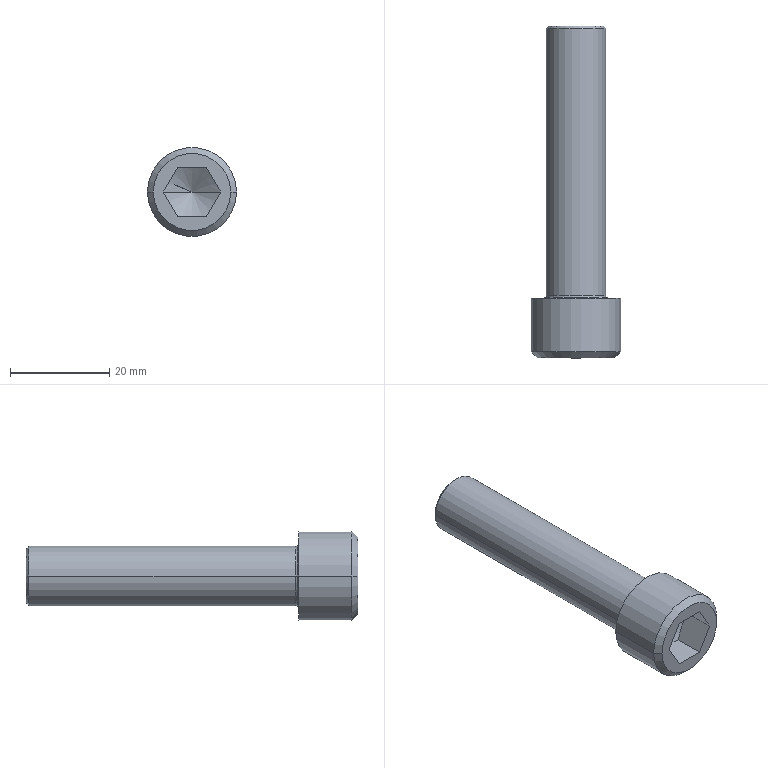Part | Creo | 1 solid | 23 faces | box 18 x 67 x 18 mm | volume 8601 mm3 | plane 9 | cone 6 | cylinder 4 | torus 4 | commonest cylinder face diameters 12 x2 18 x2
STEP:
#1=CARTESIAN_POINT('',(0.,0.,0.));
#2=DIRECTION('',(0.,0.,1.));
#3=DIRECTION('',(1.,0.,0.));
#4=AXIS2_PLACEMENT_3D('',#1,#2,#3);
#5=CARTESIAN_POINT('',(159.226,-292.,-52.5));
#6=VERTEX_POINT('',#5);
#7=CARTESIAN_POINT('',(162.113,-292.,-57.5));
#8=VERTEX_POINT('',#7);
#9=CARTESIAN_POINT('',(159.226,-292.,-52.5));
#10=CARTESIAN_POINT('',(159.361,-291.922,-52.733));
#11=CARTESIAN_POINT('',(159.631,-291.783,-53.201));
#12=CARTESIAN_POINT('',(160.043,-291.631,-53.914));
#13=CARTESIAN_POINT('',(160.46,-291.55,-54.636));
#14=CARTESIAN_POINT('',(160.878,-291.55,-55.36));
#15=CARTESIAN_POINT('',(161.296,-291.63,-56.084));
#16=CARTESIAN_POINT('',(161.707,-291.782,-56.796));
#17=CARTESIAN_POINT('',(161.978,-291.922,-57.266));
#18=CARTESIAN_POINT('',(162.113,-292.,-57.5));
#19=B_SPLINE_CURVE_WITH_KNOTS('',3,(#9,#10,#11,#12,#13,#14,#15,#16,#17,#18),.UNSPECIFIED.,.F.,.F.,(4,1,1,1,1,1,1,4),(0.,0.1429,0.2857,0.4286,0.5714,0.7143,0.8571,1.),.UNSPECIFIED.);
#20=EDGE_CURVE('',#6,#8,#19,.T.);
#21=ORIENTED_EDGE('',*,*,#20,.F.);
#22=CARTESIAN_POINT('',(165.,-288.667,-52.5));
#23=VERTEX_POINT('',#22);
#24=CARTESIAN_POINT('',(165.,-288.667,-52.5));
#25=DIRECTION('',(-0.866,-0.5,0.));
#26=VECTOR('',#25,6.667);
#27=LINE('',#24,#26);
#28=EDGE_CURVE('',#23,#6,#27,.T.);
#29=ORIENTED_EDGE('',*,*,#28,.F.);
#30=CARTESIAN_POINT('',(170.774,-292.,-52.5));
#31=VERTEX_POINT('',#30);
#32=CARTESIAN_POINT('',(165.,-288.667,-52.5));
#33=DIRECTION('',(0.866,-0.5,0.));
#34=VECTOR('',#33,6.667);
#35=LINE('',#32,#34);
#36=EDGE_CURVE('',#23,#31,#35,.T.);
#37=ORIENTED_EDGE('',*,*,#36,.T.);
#38=CARTESIAN_POINT('',(167.887,-292.,-57.5));
#39=VERTEX_POINT('',#38);
#40=CARTESIAN_POINT('',(167.887,-292.,-57.5));
#41=CARTESIAN_POINT('',(168.021,-291.922,-57.267));
#42=CARTESIAN_POINT('',(168.291,-291.783,-56.799));
#43=CARTESIAN_POINT('',(168.703,-291.631,-56.086));
#44=CARTESIAN_POINT('',(169.12,-291.55,-55.364));
#45=CARTESIAN_POINT('',(169.538,-291.55,-54.64));
#46=CARTESIAN_POINT('',(169.956,-291.63,-53.916));
#47=CARTESIAN_POINT('',(170.367,-291.782,-53.204));
#48=CARTESIAN_POINT('',(170.638,-291.922,-52.734));
#49=CARTESIAN_POINT('',(170.774,-292.,-52.5));
#50=B_SPLINE_CURVE_WITH_KNOTS('',3,(#40,#41,#42,#43,#44,#45,#46,#47,#48,#49),.UNSPECIFIED.,.F.,.F.,(4,1,1,1,1,1,1,4),(0.,0.1429,0.2857,0.4286,0.5714,0.7143,0.8571,1.),.UNSPECIFIED.);
#51=EDGE_CURVE('',#39,#31,#50,.T.);
#52=ORIENTED_EDGE('',*,*,#51,.F.);
#53=CARTESIAN_POINT('',(162.113,-292.,-57.5));
#54=CARTESIAN_POINT('',(162.381,-291.923,-57.5));
#55=CARTESIAN_POINT('',(162.919,-291.783,-57.5));
#56=CARTESIAN_POINT('',(163.745,-291.631,-57.5));
#57=CARTESIAN_POINT('',(164.581,-291.55,-57.5));
#58=CARTESIAN_POINT('',(165.416,-291.55,-57.5));
#59=CARTESIAN_POINT('',(166.25,-291.63,-57.5));
#60=CARTESIAN_POINT('',(167.077,-291.782,-57.5));
#61=CARTESIAN_POINT('',(167.618,-291.922,-57.5));
#62=CARTESIAN_POINT('',(167.887,-292.,-57.5));
#63=B_SPLINE_CURVE_WITH_KNOTS('',3,(#53,#54,#55,#56,#57,#58,#59,#60,#61,#62),.UNSPECIFIED.,.F.,.F.,(4,1,1,1,1,1,1,4),(0.,0.1429,0.2857,0.4286,0.5714,0.7143,0.8571,1.),.UNSPECIFIED.);
#64=EDGE_CURVE('',#8,#39,#63,.T.);
#65=ORIENTED_EDGE('',*,*,#64,.F.);
#66=EDGE_LOOP('',(#21,#29,#37,#52,#65));
#67=FACE_OUTER_BOUND('',#66,.F.);
#68=CARTESIAN_POINT('',(165.,-290.367,-52.5));
#69=DIRECTION('',(0.,-1.,0.));
#70=DIRECTION('',(-1.,0.,0.));
#71=AXIS2_PLACEMENT_3D('',#68,#69,#70);
#72=CONICAL_SURFACE('',#71,2.944,60.);
#73=ADVANCED_FACE('',(#67),#72,.F.);
#74=CARTESIAN_POINT('',(162.113,-298.,-57.5));
#75=VERTEX_POINT('',#74);
#76=CARTESIAN_POINT('',(159.226,-298.,-52.5));
#77=VERTEX_POINT('',#76);
#78=CARTESIAN_POINT('',(162.113,-298.,-57.5));
#79=DIRECTION('',(-0.5,0.,0.866));
#80=VECTOR('',#79,5.774);
#81=LINE('',#78,#80);
#82=EDGE_CURVE('',#75,#77,#81,.T.);
#83=ORIENTED_EDGE('',*,*,#82,.T.);
#84=CARTESIAN_POINT('',(159.226,-298.,-52.5));
#85=DIRECTION('',(0.,1.,0.));
#86=VECTOR('',#85,6.);
#87=LINE('',#84,#86);
#88=EDGE_CURVE('',#77,#6,#87,.T.);
#89=ORIENTED_EDGE('',*,*,#88,.T.);
#90=ORIENTED_EDGE('',*,*,#20,.T.);
#91=CARTESIAN_POINT('',(162.113,-298.,-57.5));
#92=DIRECTION('',(0.,1.,0.));
#93=VECTOR('',#92,6.);
#94=LINE('',#91,#93);
#95=EDGE_CURVE('',#75,#8,#94,.T.);
#96=ORIENTED_EDGE('',*,*,#95,.F.);
#97=EDGE_LOOP('',(#83,#89,#90,#96));
#98=FACE_OUTER_BOUND('',#97,.F.);
#99=CARTESIAN_POINT('',(162.113,-292.,-57.5));
#100=DIRECTION('',(0.866,0.,0.5));
#101=DIRECTION('',(-0.5,0.,0.866));
#102=AXIS2_PLACEMENT_3D('',#99,#100,#101);
#103=PLANE('',#102);
#104=ADVANCED_FACE('',(#98),#103,.T.);
#105=CARTESIAN_POINT('',(157.2,-298.,-52.5));
#106=VERTEX_POINT('',#105);
#107=CARTESIAN_POINT('',(172.8,-298.,-52.5));
#108=VERTEX_POINT('',#107);
#109=CARTESIAN_POINT('',(165.,-298.,-52.5));
#110=DIRECTION('',(0.,-1.,0.));
#111=DIRECTION('',(-1.,0.,0.));
#112=AXIS2_PLACEMENT_3D('',#109,#110,#111);
#113=CIRCLE('',#112,7.8);
#114=EDGE_CURVE('',#106,#108,#113,.T.);
#115=ORIENTED_EDGE('',*,*,#114,.F.);
#116=CARTESIAN_POINT('',(165.,-298.,-52.5));
#117=DIRECTION('',(0.,-1.,0.));
#118=DIRECTION('',(1.,0.,0.));
#119=AXIS2_PLACEMENT_3D('',#116,#117,#118);
#120=CIRCLE('',#119,7.8);
#121=EDGE_CURVE('',#108,#106,#120,.T.);
#122=ORIENTED_EDGE('',*,*,#121,.F.);
#123=EDGE_LOOP('',(#115,#122));
#124=FACE_OUTER_BOUND('',#123,.F.);
#125=CARTESIAN_POINT('',(162.113,-298.,-47.5));
#126=VERTEX_POINT('',#125);
#127=CARTESIAN_POINT('',(159.226,-298.,-52.5));
#128=DIRECTION('',(0.5,0.,0.866));
#129=VECTOR('',#128,5.774);
#130=LINE('',#127,#129);
#131=EDGE_CURVE('',#77,#126,#130,.T.);
#132=ORIENTED_EDGE('',*,*,#131,.F.);
#133=ORIENTED_EDGE('',*,*,#82,.F.);
#134=CARTESIAN_POINT('',(167.887,-298.,-57.5));
#135=VERTEX_POINT('',#134);
#136=CARTESIAN_POINT('',(162.113,-298.,-57.5));
#137=DIRECTION('',(1.,0.,0.));
#138=VECTOR('',#137,5.774);
#139=LINE('',#136,#138);
#140=EDGE_CURVE('',#75,#135,#139,.T.);
#141=ORIENTED_EDGE('',*,*,#140,.T.);
#142=CARTESIAN_POINT('',(170.774,-298.,-52.5));
#143=VERTEX_POINT('',#142);
#144=CARTESIAN_POINT('',(170.774,-298.,-52.5));
#145=DIRECTION('',(-0.5,0.,-0.866));
#146=VECTOR('',#145,5.774);
#147=LINE('',#144,#146);
#148=EDGE_CURVE('',#143,#135,#147,.T.);
#149=ORIENTED_EDGE('',*,*,#148,.F.);
#150=CARTESIAN_POINT('',(167.887,-298.,-47.5));
#151=VERTEX_POINT('',#150);
#152=CARTESIAN_POINT('',(167.887,-298.,-47.5));
#153=DIRECTION('',(0.5,0.,-0.866));
#154=VECTOR('',#153,5.774);
#155=LINE('',#152,#154);
#156=EDGE_CURVE('',#151,#143,#155,.T.);
#157=ORIENTED_EDGE('',*,*,#156,.F.);
#158=CARTESIAN_POINT('',(167.887,-298.,-47.5));
#159=DIRECTION('',(-1.,0.,0.));
#160=VECTOR('',#159,5.774);
#161=LINE('',#158,#160);
#162=EDGE_CURVE('',#151,#126,#161,.T.);
#163=ORIENTED_EDGE('',*,*,#162,.T.);
#164=EDGE_LOOP('',(#132,#133,#141,#149,#157,#163));
#165=FACE_BOUND('',#164,.F.);
#166=CARTESIAN_POINT('',(165.,-298.,-52.5));
#167=DIRECTION('',(0.,-1.,0.));
#168=DIRECTION('',(-1.,0.,0.));
#169=AXIS2_PLACEMENT_3D('',#166,#167,#168);
#170=PLANE('',#169);
#171=ADVANCED_FACE('',(#124,#165),#170,.T.);
#172=CARTESIAN_POINT('',(156.,-296.8,-52.5));
#173=VERTEX_POINT('',#172);
#174=CARTESIAN_POINT('',(174.,-296.8,-52.5));
#175=VERTEX_POINT('',#174);
#176=CARTESIAN_POINT('',(165.,-296.8,-52.5));
#177=DIRECTION('',(0.,-1.,0.));
#178=DIRECTION('',(-1.,0.,0.));
#179=AXIS2_PLACEMENT_3D('',#176,#177,#178);
#180=CIRCLE('',#179,9.);
#181=EDGE_CURVE('',#173,#175,#180,.T.);
#182=ORIENTED_EDGE('',*,*,#181,.F.);
#183=CARTESIAN_POINT('',(157.2,-298.,-52.5));
#184=DIRECTION('',(-0.7071,0.7071,0.));
#185=VECTOR('',#184,1.697);
#186=LINE('',#183,#185);
#187=EDGE_CURVE('',#106,#173,#186,.T.);
#188=ORIENTED_EDGE('',*,*,#187,.F.);
#189=ORIENTED_EDGE('',*,*,#114,.T.);
#190=CARTESIAN_POINT('',(172.8,-298.,-52.5));
#191=DIRECTION('',(0.7071,0.7071,0.));
#192=VECTOR('',#191,1.697);
#193=LINE('',#190,#192);
#194=EDGE_CURVE('',#108,#175,#193,.T.);
#195=ORIENTED_EDGE('',*,*,#194,.T.);
#196=EDGE_LOOP('',(#182,#188,#189,#195));
#197=FACE_OUTER_BOUND('',#196,.F.);
#198=CARTESIAN_POINT('',(165.,-297.4,-52.5));
#199=DIRECTION('',(0.,1.,0.));
#200=DIRECTION('',(1.,0.,0.));
#201=AXIS2_PLACEMENT_3D('',#198,#199,#200);
#202=CONICAL_SURFACE('',#201,8.4,45.);
#203=ADVANCED_FACE('',(#197),#202,.T.);
#204=ORIENTED_EDGE('',*,*,#181,.T.);
#205=CARTESIAN_POINT('',(174.,-286.,-52.5));
#206=VERTEX_POINT('',#205);
#207=CARTESIAN_POINT('',(174.,-286.,-52.5));
#208=DIRECTION('',(0.,-1.,0.));
#209=VECTOR('',#208,10.8);
#210=LINE('',#207,#209);
#211=EDGE_CURVE('',#206,#175,#210,.T.);
#212=ORIENTED_EDGE('',*,*,#211,.F.);
#213=CARTESIAN_POINT('',(156.,-286.,-52.5));
#214=VERTEX_POINT('',#213);
#215=CARTESIAN_POINT('',(165.,-286.,-52.5));
#216=DIRECTION('',(0.,1.,0.));
#217=DIRECTION('',(1.,0.,0.));
#218=AXIS2_PLACEMENT_3D('',#215,#216,#217);
#219=CIRCLE('',#218,9.);
#220=EDGE_CURVE('',#206,#214,#219,.T.);
#221=ORIENTED_EDGE('',*,*,#220,.T.);
#222=CARTESIAN_POINT('',(156.,-286.,-52.5));
#223=DIRECTION('',(0.,-1.,0.));
#224=VECTOR('',#223,10.8);
#225=LINE('',#222,#224);
#226=EDGE_CURVE('',#214,#173,#225,.T.);
#227=ORIENTED_EDGE('',*,*,#226,.T.);
#228=EDGE_LOOP('',(#204,#212,#221,#227));
#229=FACE_OUTER_BOUND('',#228,.F.);
#230=CARTESIAN_POINT('',(165.,-286.,-52.5));
#231=DIRECTION('',(0.,-1.,0.));
#232=DIRECTION('',(-1.,0.,0.));
#233=AXIS2_PLACEMENT_3D('',#230,#231,#232);
#234=CYLINDRICAL_SURFACE('',#233,9.);
#235=ADVANCED_FACE('',(#229),#234,.T.);
#236=CARTESIAN_POINT('',(165.,-296.8,-52.5));
#237=DIRECTION('',(0.,-1.,0.));
#238=DIRECTION('',(1.,0.,0.));
#239=AXIS2_PLACEMENT_3D('',#236,#237,#238);
#240=CIRCLE('',#239,9.);
#241=EDGE_CURVE('',#175,#173,#240,.T.);
#242=ORIENTED_EDGE('',*,*,#241,.T.);
#243=ORIENTED_EDGE('',*,*,#226,.F.);
#244=CARTESIAN_POINT('',(165.,-286.,-52.5));
#245=DIRECTION('',(0.,1.,0.));
#246=DIRECTION('',(-1.,0.,0.));
#247=AXIS2_PLACEMENT_3D('',#244,#245,#246);
#248=CIRCLE('',#247,9.);
#249=EDGE_CURVE('',#214,#206,#248,.T.);
#250=ORIENTED_EDGE('',*,*,#249,.T.);
#251=ORIENTED_EDGE('',*,*,#211,.T.);
#252=EDGE_LOOP('',(#242,#243,#250,#251));
#253=FACE_OUTER_BOUND('',#252,.F.);
#254=CARTESIAN_POINT('',(165.,-286.,-52.5));
#255=DIRECTION('',(0.,-1.,0.));
#256=DIRECTION('',(-1.,0.,0.));
#257=AXIS2_PLACEMENT_3D('',#254,#255,#256);
#258=CYLINDRICAL_SURFACE('',#257,9.);
#259=ADVANCED_FACE('',(#253),#258,.T.);
#260=ORIENTED_EDGE('',*,*,#241,.F.);
#261=ORIENTED_EDGE('',*,*,#194,.F.);
#262=ORIENTED_EDGE('',*,*,#121,.T.);
#263=ORIENTED_EDGE('',*,*,#187,.T.);
#264=EDGE_LOOP('',(#260,#261,#262,#263));
#265=FACE_OUTER_BOUND('',#264,.F.);
#266=CARTESIAN_POINT('',(165.,-297.4,-52.5));
#267=DIRECTION('',(0.,1.,0.));
#268=DIRECTION('',(1.,0.,0.));
#269=AXIS2_PLACEMENT_3D('',#266,#267,#268);
#270=CONICAL_SURFACE('',#269,8.4,45.);
#271=ADVANCED_FACE('',(#265),#270,.T.);
#272=ORIENTED_EDGE('',*,*,#249,.F.);
#273=ORIENTED_EDGE('',*,*,#220,.F.);
#274=EDGE_LOOP('',(#272,#273));
#275=FACE_OUTER_BOUND('',#274,.F.);
#276=CARTESIAN_POINT('',(158.4,-286.,-52.5));
#277=VERTEX_POINT('',#276);
#278=CARTESIAN_POINT('',(171.6,-286.,-52.5));
#279=VERTEX_POINT('',#278);
#280=CARTESIAN_POINT('',(165.,-286.,-52.5));
#281=DIRECTION('',(0.,-1.,0.));
#282=DIRECTION('',(-1.,0.,0.));
#283=AXIS2_PLACEMENT_3D('',#280,#281,#282);
#284=CIRCLE('',#283,6.6);
#285=EDGE_CURVE('',#277,#279,#284,.T.);
#286=ORIENTED_EDGE('',*,*,#285,.F.);
#287=CARTESIAN_POINT('',(165.,-286.,-52.5));
#288=DIRECTION('',(0.,-1.,0.));
#289=DIRECTION('',(1.,0.,0.));
#290=AXIS2_PLACEMENT_3D('',#287,#288,#289);
#291=CIRCLE('',#290,6.6);
#292=EDGE_CURVE('',#279,#277,#291,.T.);
#293=ORIENTED_EDGE('',*,*,#292,.F.);
#294=EDGE_LOOP('',(#286,#293));
#295=FACE_BOUND('',#294,.F.);
#296=CARTESIAN_POINT('',(165.,-286.,-52.5));
#297=DIRECTION('',(0.,-1.,0.));
#298=DIRECTION('',(-1.,0.,0.));
#299=AXIS2_PLACEMENT_3D('',#296,#297,#298);
#300=PLANE('',#299);
#301=ADVANCED_FACE('',(#275,#295),#300,.F.);
#302=ORIENTED_EDGE('',*,*,#285,.T.);
#303=CARTESIAN_POINT('',(171.176,-285.824,-52.5));
#304=VERTEX_POINT('',#303);
#305=CARTESIAN_POINT('',(171.6,-285.4,-52.5));
#306=DIRECTION('',(0.,0.,-1.));
#307=DIRECTION('',(0.,-1.,0.));
#308=AXIS2_PLACEMENT_3D('',#305,#306,#307);
#309=CIRCLE('',#308,0.6);
#310=EDGE_CURVE('',#279,#304,#309,.T.);
#311=ORIENTED_EDGE('',*,*,#310,.T.);
#312=CARTESIAN_POINT('',(158.824,-285.824,-52.5));
#313=VERTEX_POINT('',#312);
#314=CARTESIAN_POINT('',(165.,-285.824,-52.5));
#315=DIRECTION('',(0.,-1.,0.));
#316=DIRECTION('',(-1.,0.,0.));
#317=AXIS2_PLACEMENT_3D('',#314,#315,#316);
#318=CIRCLE('',#317,6.176);
#319=EDGE_CURVE('',#313,#304,#318,.T.);
#320=ORIENTED_EDGE('',*,*,#319,.F.);
#321=CARTESIAN_POINT('',(158.4,-285.4,-52.5));
#322=DIRECTION('',(0.,0.,1.));
#323=DIRECTION('',(0.,-1.,0.));
#324=AXIS2_PLACEMENT_3D('',#321,#322,#323);
#325=CIRCLE('',#324,0.6);
#326=EDGE_CURVE('',#277,#313,#325,.T.);
#327=ORIENTED_EDGE('',*,*,#326,.F.);
#328=EDGE_LOOP('',(#302,#311,#320,#327));
#329=FACE_OUTER_BOUND('',#328,.F.);
#330=CARTESIAN_POINT('',(165.,-285.4,-52.5));
#331=DIRECTION('',(0.,-1.,0.));
#332=DIRECTION('',(-1.,0.,0.));
#333=AXIS2_PLACEMENT_3D('',#330,#331,#332);
#334=TOROIDAL_SURFACE('',#333,6.6,0.6);
#335=ADVANCED_FACE('',(#329),#334,.F.);
#336=ORIENTED_EDGE('',*,*,#292,.T.);
#337=ORIENTED_EDGE('',*,*,#326,.T.);
#338=CARTESIAN_POINT('',(165.,-285.824,-52.5));
#339=DIRECTION('',(0.,-1.,0.));
#340=DIRECTION('',(1.,0.,0.));
#341=AXIS2_PLACEMENT_3D('',#338,#339,#340);
#342=CIRCLE('',#341,6.176);
#343=EDGE_CURVE('',#304,#313,#342,.T.);
#344=ORIENTED_EDGE('',*,*,#343,.F.);
#345=ORIENTED_EDGE('',*,*,#310,.F.);
#346=EDGE_LOOP('',(#336,#337,#344,#345));
#347=FACE_OUTER_BOUND('',#346,.F.);
#348=CARTESIAN_POINT('',(165.,-285.4,-52.5));
#349=DIRECTION('',(0.,-1.,0.));
#350=DIRECTION('',(-1.,0.,0.));
#351=AXIS2_PLACEMENT_3D('',#348,#349,#350);
#352=TOROIDAL_SURFACE('',#351,6.6,0.6);
#353=ADVANCED_FACE('',(#347),#352,.F.);
#354=CARTESIAN_POINT('',(171.,-285.4,-52.5));
#355=VERTEX_POINT('',#354);
#356=CARTESIAN_POINT('',(159.,-285.4,-52.5));
#357=VERTEX_POINT('',#356);
#358=CARTESIAN_POINT('',(165.,-285.4,-52.5));
#359=DIRECTION('',(0.,-1.,0.));
#360=DIRECTION('',(1.,0.,0.));
#361=AXIS2_PLACEMENT_3D('',#358,#359,#360);
#362=CIRCLE('',#361,6.);
#363=EDGE_CURVE('',#355,#357,#362,.T.);
#364=ORIENTED_EDGE('',*,*,#363,.F.);
#365=CARTESIAN_POINT('',(171.6,-285.4,-52.5));
#366=DIRECTION('',(0.,0.,-1.));
#367=DIRECTION('',(-0.7071,-0.7071,0.));
#368=AXIS2_PLACEMENT_3D('',#365,#366,#367);
#369=CIRCLE('',#368,0.6);
#370=EDGE_CURVE('',#304,#355,#369,.T.);
#371=ORIENTED_EDGE('',*,*,#370,.F.);
#372=ORIENTED_EDGE('',*,*,#343,.T.);
#373=CARTESIAN_POINT('',(158.4,-285.4,-52.5));
#374=DIRECTION('',(0.,0.,1.));
#375=DIRECTION('',(0.7071,-0.7071,0.));
#376=AXIS2_PLACEMENT_3D('',#373,#374,#375);
#377=CIRCLE('',#376,0.6);
#378=EDGE_CURVE('',#313,#357,#377,.T.);
#379=ORIENTED_EDGE('',*,*,#378,.T.);
#380=EDGE_LOOP('',(#364,#371,#372,#379));
#381=FACE_OUTER_BOUND('',#380,.F.);
#382=CARTESIAN_POINT('',(165.,-285.4,-52.5));
#383=DIRECTION('',(0.,-1.,0.));
#384=DIRECTION('',(-1.,0.,0.));
#385=AXIS2_PLACEMENT_3D('',#382,#383,#384);
#386=TOROIDAL_SURFACE('',#385,6.6,0.6);
#387=ADVANCED_FACE('',(#381),#386,.F.);
#388=CARTESIAN_POINT('',(159.,-231.5,-52.5));
#389=VERTEX_POINT('',#388);
#390=CARTESIAN_POINT('',(171.,-231.5,-52.5));
#391=VERTEX_POINT('',#390);
#392=CARTESIAN_POINT('',(165.,-231.5,-52.5));
#393=DIRECTION('',(0.,1.,0.));
#394=DIRECTION('',(-1.,0.,0.));
#395=AXIS2_PLACEMENT_3D('',#392,#393,#394);
#396=CIRCLE('',#395,6.);
#397=EDGE_CURVE('',#389,#391,#396,.T.);
#398=ORIENTED_EDGE('',*,*,#397,.T.);
#399=CARTESIAN_POINT('',(171.,-231.5,-52.5));
#400=DIRECTION('',(0.,-1.,0.));
#401=VECTOR('',#400,53.9);
#402=LINE('',#399,#401);
#403=EDGE_CURVE('',#391,#355,#402,.T.);
#404=ORIENTED_EDGE('',*,*,#403,.T.);
#405=ORIENTED_EDGE('',*,*,#363,.T.);
#406=CARTESIAN_POINT('',(159.,-231.5,-52.5));
#407=DIRECTION('',(0.,-1.,0.));
#408=VECTOR('',#407,53.9);
#409=LINE('',#406,#408);
#410=EDGE_CURVE('',#389,#357,#409,.T.);
#411=ORIENTED_EDGE('',*,*,#410,.F.);
#412=EDGE_LOOP('',(#398,#404,#405,#411));
#413=FACE_OUTER_BOUND('',#412,.F.);
#414=CARTESIAN_POINT('',(165.,-231.,-52.5));
#415=DIRECTION('',(0.,-1.,0.));
#416=DIRECTION('',(-1.,0.,0.));
#417=AXIS2_PLACEMENT_3D('',#414,#415,#416);
#418=CYLINDRICAL_SURFACE('',#417,6.);
#419=ADVANCED_FACE('',(#413),#418,.T.);
#420=CARTESIAN_POINT('',(159.5,-231.,-52.5));
#421=VERTEX_POINT('',#420);
#422=CARTESIAN_POINT('',(170.5,-231.,-52.5));
#423=VERTEX_POINT('',#422);
#424=CARTESIAN_POINT('',(165.,-231.,-52.5));
#425=DIRECTION('',(0.,1.,0.));
#426=DIRECTION('',(-1.,0.,0.));
#427=AXIS2_PLACEMENT_3D('',#424,#425,#426);
#428=CIRCLE('',#427,5.5);
#429=EDGE_CURVE('',#421,#423,#428,.T.);
#430=ORIENTED_EDGE('',*,*,#429,.T.);
#431=CARTESIAN_POINT('',(170.5,-231.,-52.5));
#432=DIRECTION('',(0.7071,-0.7071,0.));
#433=VECTOR('',#432,0.7071);
#434=LINE('',#431,#433);
#435=EDGE_CURVE('',#423,#391,#434,.T.);
#436=ORIENTED_EDGE('',*,*,#435,.T.);
#437=ORIENTED_EDGE('',*,*,#397,.F.);
#438=CARTESIAN_POINT('',(159.5,-231.,-52.5));
#439=DIRECTION('',(-0.7071,-0.7071,0.));
#440=VECTOR('',#439,0.7071);
#441=LINE('',#438,#440);
#442=EDGE_CURVE('',#421,#389,#441,.T.);
#443=ORIENTED_EDGE('',*,*,#442,.F.);
#444=EDGE_LOOP('',(#430,#436,#437,#443));
#445=FACE_OUTER_BOUND('',#444,.F.);
#446=CARTESIAN_POINT('',(165.,-231.25,-52.5));
#447=DIRECTION('',(0.,-1.,0.));
#448=DIRECTION('',(-1.,0.,0.));
#449=AXIS2_PLACEMENT_3D('',#446,#447,#448);
#450=CONICAL_SURFACE('',#449,5.75,45.);
#451=ADVANCED_FACE('',(#445),#450,.T.);
#452=ORIENTED_EDGE('',*,*,#429,.F.);
#453=CARTESIAN_POINT('',(165.,-231.,-52.5));
#454=DIRECTION('',(0.,1.,0.));
#455=DIRECTION('',(1.,0.,0.));
#456=AXIS2_PLACEMENT_3D('',#453,#454,#455);
#457=CIRCLE('',#456,5.5);
#458=EDGE_CURVE('',#423,#421,#457,.T.);
#459=ORIENTED_EDGE('',*,*,#458,.F.);
#460=EDGE_LOOP('',(#452,#459));
#461=FACE_OUTER_BOUND('',#460,.F.);
#462=CARTESIAN_POINT('',(165.,-231.,-52.5));
#463=DIRECTION('',(0.,-1.,0.));
#464=DIRECTION('',(-1.,0.,0.));
#465=AXIS2_PLACEMENT_3D('',#462,#463,#464);
#466=PLANE('',#465);
#467=ADVANCED_FACE('',(#461),#466,.F.);
#468=ORIENTED_EDGE('',*,*,#458,.T.);
#469=ORIENTED_EDGE('',*,*,#442,.T.);
#470=CARTESIAN_POINT('',(165.,-231.5,-52.5));
#471=DIRECTION('',(0.,1.,0.));
#472=DIRECTION('',(1.,0.,0.));
#473=AXIS2_PLACEMENT_3D('',#470,#471,#472);
#474=CIRCLE('',#473,6.);
#475=EDGE_CURVE('',#391,#389,#474,.T.);
#476=ORIENTED_EDGE('',*,*,#475,.F.);
#477=ORIENTED_EDGE('',*,*,#435,.F.);
#478=EDGE_LOOP('',(#468,#469,#476,#477));
#479=FACE_OUTER_BOUND('',#478,.F.);
#480=CARTESIAN_POINT('',(165.,-231.25,-52.5));
#481=DIRECTION('',(0.,-1.,0.));
#482=DIRECTION('',(-1.,0.,0.));
#483=AXIS2_PLACEMENT_3D('',#480,#481,#482);
#484=CONICAL_SURFACE('',#483,5.75,45.);
#485=ADVANCED_FACE('',(#479),#484,.T.);
#486=ORIENTED_EDGE('',*,*,#475,.T.);
#487=ORIENTED_EDGE('',*,*,#410,.T.);
#488=CARTESIAN_POINT('',(165.,-285.4,-52.5));
#489=DIRECTION('',(0.,-1.,0.));
#490=DIRECTION('',(-1.,0.,0.));
#491=AXIS2_PLACEMENT_3D('',#488,#489,#490);
#492=CIRCLE('',#491,6.);
#493=EDGE_CURVE('',#357,#355,#492,.T.);
#494=ORIENTED_EDGE('',*,*,#493,.T.);
#495=ORIENTED_EDGE('',*,*,#403,.F.);
#496=EDGE_LOOP('',(#486,#487,#494,#495));
#497=FACE_OUTER_BOUND('',#496,.F.);
#498=CARTESIAN_POINT('',(165.,-231.,-52.5));
#499=DIRECTION('',(0.,-1.,0.));
#500=DIRECTION('',(-1.,0.,0.));
#501=AXIS2_PLACEMENT_3D('',#498,#499,#500);
#502=CYLINDRICAL_SURFACE('',#501,6.);
#503=ADVANCED_FACE('',(#497),#502,.T.);
#504=ORIENTED_EDGE('',*,*,#493,.F.);
#505=ORIENTED_EDGE('',*,*,#378,.F.);
#506=ORIENTED_EDGE('',*,*,#319,.T.);
#507=ORIENTED_EDGE('',*,*,#370,.T.);
#508=EDGE_LOOP('',(#504,#505,#506,#507));
#509=FACE_OUTER_BOUND('',#508,.F.);
#510=CARTESIAN_POINT('',(165.,-285.4,-52.5));
#511=DIRECTION('',(0.,-1.,0.));
#512=DIRECTION('',(-1.,0.,0.));
#513=AXIS2_PLACEMENT_3D('',#510,#511,#512);
#514=TOROIDAL_SURFACE('',#513,6.6,0.6);
#515=ADVANCED_FACE('',(#509),#514,.F.);
#516=ORIENTED_EDGE('',*,*,#131,.T.);
#517=CARTESIAN_POINT('',(162.113,-292.,-47.5));
#518=VERTEX_POINT('',#517);
#519=CARTESIAN_POINT('',(162.113,-298.,-47.5));
#520=DIRECTION('',(0.,1.,0.));
#521=VECTOR('',#520,6.);
#522=LINE('',#519,#521);
#523=EDGE_CURVE('',#126,#518,#522,.T.);
#524=ORIENTED_EDGE('',*,*,#523,.T.);
#525=CARTESIAN_POINT('',(162.113,-292.,-47.5));
#526=CARTESIAN_POINT('',(161.979,-291.922,-47.733));
#527=CARTESIAN_POINT('',(161.709,-291.783,-48.201));
#528=CARTESIAN_POINT('',(161.297,-291.631,-48.914));
#529=CARTESIAN_POINT('',(160.88,-291.55,-49.636));
#530=CARTESIAN_POINT('',(160.462,-291.55,-50.36));
#531=CARTESIAN_POINT('',(160.044,-291.63,-51.084));
#532=CARTESIAN_POINT('',(159.633,-291.782,-51.796));
#533=CARTESIAN_POINT('',(159.362,-291.922,-52.266));
#534=CARTESIAN_POINT('',(159.226,-292.,-52.5));
#535=B_SPLINE_CURVE_WITH_KNOTS('',3,(#525,#526,#527,#528,#529,#530,#531,#532,#533,#534),.UNSPECIFIED.,.F.,.F.,(4,1,1,1,1,1,1,4),(0.,0.1429,0.2857,0.4286,0.5714,0.7143,0.8571,1.),.UNSPECIFIED.);
#536=EDGE_CURVE('',#518,#6,#535,.T.);
#537=ORIENTED_EDGE('',*,*,#536,.T.);
#538=ORIENTED_EDGE('',*,*,#88,.F.);
#539=EDGE_LOOP('',(#516,#524,#537,#538));
#540=FACE_OUTER_BOUND('',#539,.F.);
#541=CARTESIAN_POINT('',(159.226,-292.,-52.5));
#542=DIRECTION('',(0.866,0.,-0.5));
#543=DIRECTION('',(0.5,0.,0.866));
#544=AXIS2_PLACEMENT_3D('',#541,#542,#543);
#545=PLANE('',#544);
#546=ADVANCED_FACE('',(#540),#545,.T.);
#547=ORIENTED_EDGE('',*,*,#162,.F.);
#548=CARTESIAN_POINT('',(167.887,-292.,-47.5));
#549=VERTEX_POINT('',#548);
#550=CARTESIAN_POINT('',(167.887,-298.,-47.5));
#551=DIRECTION('',(0.,1.,0.));
#552=VECTOR('',#551,6.);
#553=LINE('',#550,#552);
#554=EDGE_CURVE('',#151,#549,#553,.T.);
#555=ORIENTED_EDGE('',*,*,#554,.T.);
#556=CARTESIAN_POINT('',(167.887,-292.,-47.5));
#557=CARTESIAN_POINT('',(167.618,-291.922,-47.5));
#558=CARTESIAN_POINT('',(167.077,-291.782,-47.5));
#559=CARTESIAN_POINT('',(166.25,-291.63,-47.5));
#560=CARTESIAN_POINT('',(165.416,-291.55,-47.5));
#561=CARTESIAN_POINT('',(164.581,-291.55,-47.5));
#562=CARTESIAN_POINT('',(163.745,-291.631,-47.5));
#563=CARTESIAN_POINT('',(162.919,-291.783,-47.5));
#564=CARTESIAN_POINT('',(162.381,-291.923,-47.5));
#565=CARTESIAN_POINT('',(162.113,-292.,-47.5));
#566=B_SPLINE_CURVE_WITH_KNOTS('',3,(#556,#557,#558,#559,#560,#561,#562,#563,#564,#565),.UNSPECIFIED.,.F.,.F.,(4,1,1,1,1,1,1,4),(0.,0.1429,0.2857,0.4286,0.5714,0.7143,0.8571,1.),.UNSPECIFIED.);
#567=EDGE_CURVE('',#549,#518,#566,.T.);
#568=ORIENTED_EDGE('',*,*,#567,.T.);
#569=ORIENTED_EDGE('',*,*,#523,.F.);
#570=EDGE_LOOP('',(#547,#555,#568,#569));
#571=FACE_OUTER_BOUND('',#570,.F.);
#572=CARTESIAN_POINT('',(162.113,-292.,-47.5));
#573=DIRECTION('',(0.,0.,-1.));
#574=DIRECTION('',(0.,-1.,0.));
#575=AXIS2_PLACEMENT_3D('',#572,#573,#574);
#576=PLANE('',#575);
#577=ADVANCED_FACE('',(#571),#576,.T.);
#578=ORIENTED_EDGE('',*,*,#156,.T.);
#579=CARTESIAN_POINT('',(170.774,-298.,-52.5));
#580=DIRECTION('',(0.,1.,0.));
#581=VECTOR('',#580,6.);
#582=LINE('',#579,#581);
#583=EDGE_CURVE('',#143,#31,#582,.T.);
#584=ORIENTED_EDGE('',*,*,#583,.T.);
#585=CARTESIAN_POINT('',(170.774,-292.,-52.5));
#586=CARTESIAN_POINT('',(170.638,-291.922,-52.266));
#587=CARTESIAN_POINT('',(170.367,-291.782,-51.796));
#588=CARTESIAN_POINT('',(169.956,-291.63,-51.084));
#589=CARTESIAN_POINT('',(169.538,-291.55,-50.36));
#590=CARTESIAN_POINT('',(169.12,-291.55,-49.636));
#591=CARTESIAN_POINT('',(168.703,-291.631,-48.914));
#592=CARTESIAN_POINT('',(168.291,-291.783,-48.201));
#593=CARTESIAN_POINT('',(168.021,-291.922,-47.733));
#594=CARTESIAN_POINT('',(167.887,-292.,-47.5));
#595=B_SPLINE_CURVE_WITH_KNOTS('',3,(#585,#586,#587,#588,#589,#590,#591,#592,#593,#594),.UNSPECIFIED.,.F.,.F.,(4,1,1,1,1,1,1,4),(0.,0.1429,0.2857,0.4286,0.5714,0.7143,0.8571,1.),.UNSPECIFIED.);
#596=EDGE_CURVE('',#31,#549,#595,.T.);
#597=ORIENTED_EDGE('',*,*,#596,.T.);
#598=ORIENTED_EDGE('',*,*,#554,.F.);
#599=EDGE_LOOP('',(#578,#584,#597,#598));
#600=FACE_OUTER_BOUND('',#599,.F.);
#601=CARTESIAN_POINT('',(167.887,-292.,-47.5));
#602=DIRECTION('',(-0.866,0.,-0.5));
#603=DIRECTION('',(0.5,0.,-0.866));
#604=AXIS2_PLACEMENT_3D('',#601,#602,#603);
#605=PLANE('',#604);
#606=ADVANCED_FACE('',(#600),#605,.T.);
#607=ORIENTED_EDGE('',*,*,#148,.T.);
#608=CARTESIAN_POINT('',(167.887,-298.,-57.5));
#609=DIRECTION('',(0.,1.,0.));
#610=VECTOR('',#609,6.);
#611=LINE('',#608,#610);
#612=EDGE_CURVE('',#135,#39,#611,.T.);
#613=ORIENTED_EDGE('',*,*,#612,.T.);
#614=ORIENTED_EDGE('',*,*,#51,.T.);
#615=ORIENTED_EDGE('',*,*,#583,.F.);
#616=EDGE_LOOP('',(#607,#613,#614,#615));
#617=FACE_OUTER_BOUND('',#616,.F.);
#618=CARTESIAN_POINT('',(170.774,-292.,-52.5));
#619=DIRECTION('',(-0.866,0.,0.5));
#620=DIRECTION('',(-0.5,0.,-0.866));
#621=AXIS2_PLACEMENT_3D('',#618,#619,#620);
#622=PLANE('',#621);
#623=ADVANCED_FACE('',(#617),#622,.T.);
#624=ORIENTED_EDGE('',*,*,#140,.F.);
#625=ORIENTED_EDGE('',*,*,#95,.T.);
#626=ORIENTED_EDGE('',*,*,#64,.T.);
#627=ORIENTED_EDGE('',*,*,#612,.F.);
#628=EDGE_LOOP('',(#624,#625,#626,#627));
#629=FACE_OUTER_BOUND('',#628,.F.);
#630=CARTESIAN_POINT('',(167.887,-292.,-57.5));
#631=DIRECTION('',(0.,0.,1.));
#632=DIRECTION('',(0.,1.,0.));
#633=AXIS2_PLACEMENT_3D('',#630,#631,#632);
#634=PLANE('',#633);
#635=ADVANCED_FACE('',(#629),#634,.T.);
#636=ORIENTED_EDGE('',*,*,#596,.F.);
#637=ORIENTED_EDGE('',*,*,#36,.F.);
#638=ORIENTED_EDGE('',*,*,#28,.T.);
#639=ORIENTED_EDGE('',*,*,#536,.F.);
#640=ORIENTED_EDGE('',*,*,#567,.F.);
#641=EDGE_LOOP('',(#636,#637,#638,#639,#640));
#642=FACE_OUTER_BOUND('',#641,.F.);
#643=CARTESIAN_POINT('',(165.,-290.367,-52.5));
#644=DIRECTION('',(0.,-1.,0.));
#645=DIRECTION('',(-1.,0.,0.));
#646=AXIS2_PLACEMENT_3D('',#643,#644,#645);
#647=CONICAL_SURFACE('',#646,2.944,60.);
#648=ADVANCED_FACE('',(#642),#647,.F.);
#649=CLOSED_SHELL('',(#73,#104,#171,#203,#235,#259,#271,#301,#335,#353,#387,#419,#451,#467,#485,#503,#515,#546,#577,#606,#623,#635,#648));
#650=MANIFOLD_SOLID_BREP('',#649);
#651=(LENGTH_UNIT()NAMED_UNIT(*)SI_UNIT(.MILLI.,.METRE.));
#652=UNCERTAINTY_MEASURE_WITH_UNIT(LENGTH_MEASURE(0.007167),#651,'','');
#653=(NAMED_UNIT(*)PLANE_ANGLE_UNIT()SI_UNIT($,.RADIAN.));
#654=PLANE_ANGLE_MEASURE_WITH_UNIT(PLANE_ANGLE_MEASURE(0.01745),#653);
#655=(CONVERSION_BASED_UNIT('DEGREE',#654)NAMED_UNIT(*)PLANE_ANGLE_UNIT());
#656=(NAMED_UNIT(*)SI_UNIT($,.STERADIAN.)SOLID_ANGLE_UNIT());
#657=(GEOMETRIC_REPRESENTATION_CONTEXT(3)GLOBAL_UNCERTAINTY_ASSIGNED_CONTEXT((#652))GLOBAL_UNIT_ASSIGNED_CONTEXT((#651,#655,#656))REPRESENTATION_CONTEXT('',''));
#658=ADVANCED_BREP_SHAPE_REPRESENTATION('',(#4,#650),#657);